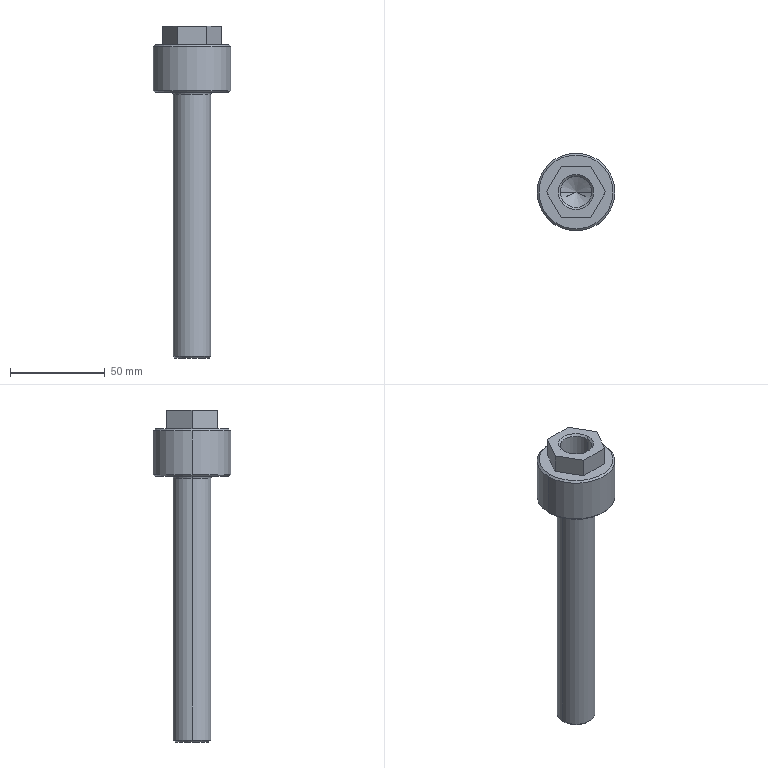Part | STEP file | YCD14007A-08.02.06-Extension Adjusting Rod-A4 | 1 solid | 28 faces | box 41 x 41 x 175 mm | volume 76364 mm3 | cone 10 | plane 10 | cylinder 6 | torus 2 | commonest cylinder face diameters 16.5 x2 20 x2 41 x2